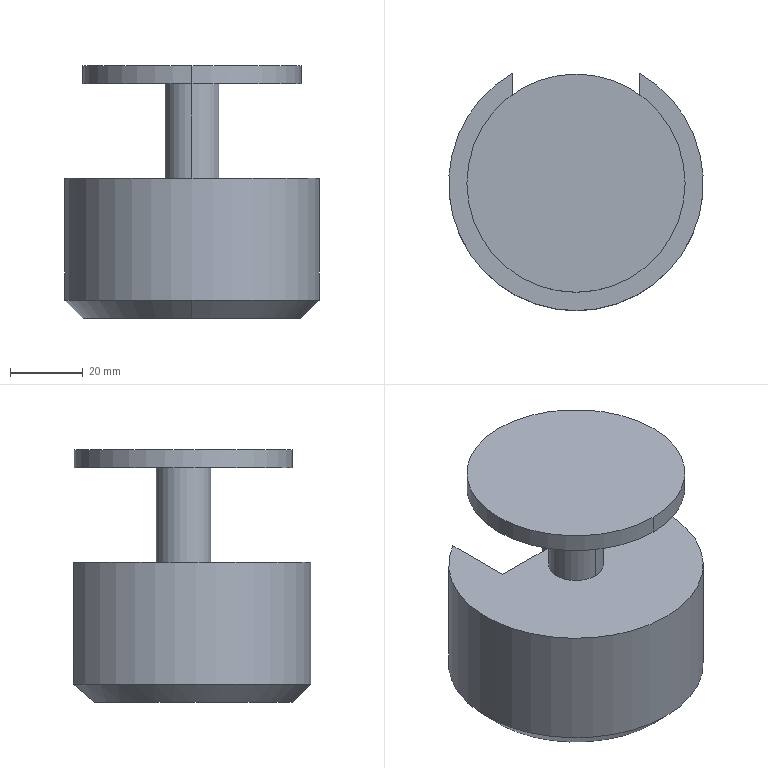Part | STEP file | ASND-0110-E63-HLTP01Clogo.sldasm-Part-213 | 1 solid | 14 faces | box 70 x 65.311 x 69.5 mm | volume 134446 mm3 | plane 7 | cylinder 5 | cone 2 | commonest cylinder face diameters 15 x2 60 x2 70 x1
STEP:
#1=CARTESIAN_POINT('',(0.,0.,0.));
#2=DIRECTION('',(0.,0.,1.));
#3=DIRECTION('',(1.,0.,0.));
#4=AXIS2_PLACEMENT_3D('',#1,#2,#3);
#5=CARTESIAN_POINT('',(320.5,-90.,-1064.2));
#6=VERTEX_POINT('',#5);
#7=CARTESIAN_POINT('',(303.,-35.633,-1064.2));
#8=VERTEX_POINT('',#7);
#9=CARTESIAN_POINT('',(320.5,-60.,-1064.2));
#10=DIRECTION('',(0.,0.,-1.));
#11=DIRECTION('',(0.,1.,0.));
#12=AXIS2_PLACEMENT_3D('',#9,#10,#11);
#13=CIRCLE('',#12,30.);
#14=CARTESIAN_POINT('',(320.5,-60.,-1064.2));
#15=DIRECTION('',(0.,0.,1.));
#16=DIRECTION('',(0.,-1.,0.));
#17=AXIS2_PLACEMENT_3D('',#14,#15,#16);
#18=CONICAL_SURFACE('',#17,30.,0.7854);
#19=CARTESIAN_POINT('',(9.425,0.));
#20=DIRECTION('',(-1.,0.));
#21=VECTOR('',#20,1.);
#22=LINE('',#19,#21);
#23=(GEOMETRIC_REPRESENTATION_CONTEXT(2)PARAMETRIC_REPRESENTATION_CONTEXT()REPRESENTATION_CONTEXT('',''));
#24=DEFINITIONAL_REPRESENTATION('',(#22),#23);
#25=PCURVE('',#18,#24);
#26=CARTESIAN_POINT('',(320.5,-60.,-1064.2));
#27=DIRECTION('',(0.,0.,-1.));
#28=DIRECTION('',(0.7071,0.7071,0.));
#29=AXIS2_PLACEMENT_3D('',#26,#27,#28);
#30=PLANE('',#29);
#31=CARTESIAN_POINT('',(0.,0.));
#32=DIRECTION('',(0.7071,-0.7071));
#33=AXIS2_PLACEMENT_2D('',#31,#32);
#34=CIRCLE('',#33,30.);
#35=(GEOMETRIC_REPRESENTATION_CONTEXT(2)PARAMETRIC_REPRESENTATION_CONTEXT()REPRESENTATION_CONTEXT('',''));
#36=DEFINITIONAL_REPRESENTATION('',(#34),#35);
#37=PCURVE('',#30,#36);
#38=SURFACE_CURVE('',#13,(#25,#37),.PCURVE_S1.);
#39=EDGE_CURVE('',#6,#8,#38,.T.);
#40=ORIENTED_EDGE('',*,*,#39,.F.);
#41=CARTESIAN_POINT('',(320.5,-95.,-1059.2));
#42=VERTEX_POINT('',#41);
#43=CARTESIAN_POINT('',(320.5,-90.,-1064.2));
#44=DIRECTION('',(0.,-0.7071,0.7071));
#45=VECTOR('',#44,1.);
#46=LINE('',#43,#45);
#47=CARTESIAN_POINT('',(6.283,0.));
#48=DIRECTION('',(0.,1.));
#49=VECTOR('',#48,1.);
#50=LINE('',#47,#49);
#51=(GEOMETRIC_REPRESENTATION_CONTEXT(2)PARAMETRIC_REPRESENTATION_CONTEXT()REPRESENTATION_CONTEXT('',''));
#52=DEFINITIONAL_REPRESENTATION('',(#50),#51);
#53=PCURVE('',#18,#52);
#54=CARTESIAN_POINT('',(320.5,-60.,-1064.2));
#55=DIRECTION('',(0.,0.,1.));
#56=DIRECTION('',(0.,-1.,0.));
#57=AXIS2_PLACEMENT_3D('',#54,#55,#56);
#58=CONICAL_SURFACE('',#57,30.,0.7854);
#59=CARTESIAN_POINT('',(0.,0.));
#60=DIRECTION('',(0.,1.));
#61=VECTOR('',#60,1.);
#62=LINE('',#59,#61);
#63=(GEOMETRIC_REPRESENTATION_CONTEXT(2)PARAMETRIC_REPRESENTATION_CONTEXT()REPRESENTATION_CONTEXT('',''));
#64=DEFINITIONAL_REPRESENTATION('',(#62),#63);
#65=PCURVE('',#58,#64);
#66=SURFACE_CURVE('',#46,(#53,#65),.PCURVE_S1.);
#67=EDGE_CURVE('',#6,#42,#66,.T.);
#68=ORIENTED_EDGE('',*,*,#67,.T.);
#69=CARTESIAN_POINT('',(303.,-29.689,-1059.2));
#70=VERTEX_POINT('',#69);
#71=CARTESIAN_POINT('',(320.5,-60.,-1059.2));
#72=DIRECTION('',(0.,0.,1.));
#73=DIRECTION('',(0.,1.,0.));
#74=AXIS2_PLACEMENT_3D('',#71,#72,#73);
#75=CIRCLE('',#74,35.);
#76=CARTESIAN_POINT('',(3.142,5.));
#77=DIRECTION('',(1.,0.));
#78=VECTOR('',#77,1.);
#79=LINE('',#76,#78);
#80=(GEOMETRIC_REPRESENTATION_CONTEXT(2)PARAMETRIC_REPRESENTATION_CONTEXT()REPRESENTATION_CONTEXT('',''));
#81=DEFINITIONAL_REPRESENTATION('',(#79),#80);
#82=PCURVE('',#18,#81);
#83=CARTESIAN_POINT('',(320.5,-60.,-1025.7));
#84=DIRECTION('',(0.,0.,-1.));
#85=DIRECTION('',(0.,1.,0.));
#86=AXIS2_PLACEMENT_3D('',#83,#84,#85);
#87=CYLINDRICAL_SURFACE('',#86,35.);
#88=CARTESIAN_POINT('',(6.283,33.5));
#89=DIRECTION('',(-1.,0.));
#90=VECTOR('',#89,1.);
#91=LINE('',#88,#90);
#92=(GEOMETRIC_REPRESENTATION_CONTEXT(2)PARAMETRIC_REPRESENTATION_CONTEXT()REPRESENTATION_CONTEXT('',''));
#93=DEFINITIONAL_REPRESENTATION('',(#91),#92);
#94=PCURVE('',#87,#93);
#95=SURFACE_CURVE('',#75,(#82,#94),.PCURVE_S1.);
#96=EDGE_CURVE('',#70,#42,#95,.T.);
#97=ORIENTED_EDGE('',*,*,#96,.F.);
#98=CARTESIAN_POINT('',(303.,-35.633,-1064.2));
#99=CARTESIAN_POINT('',(303.,-32.89,-1061.972));
#100=CARTESIAN_POINT('',(303.,-29.689,-1059.2));
#101=(BOUNDED_CURVE()B_SPLINE_CURVE(2,(#98,#99,#100),.UNSPECIFIED.,.F.,.F.)B_SPLINE_CURVE_WITH_KNOTS((3,3),(0.253,1.379),.PIECEWISE_BEZIER_KNOTS.)CURVE()GEOMETRIC_REPRESENTATION_ITEM()RATIONAL_B_SPLINE_CURVE((1.01,1.03,1.042))REPRESENTATION_ITEM(''));
#102=CARTESIAN_POINT('',(3.764,0.));
#103=CARTESIAN_POINT('',(3.763,0.06889));
#104=CARTESIAN_POINT('',(3.759,0.2073));
#105=CARTESIAN_POINT('',(3.755,0.4166));
#106=CARTESIAN_POINT('',(3.75,0.6277));
#107=CARTESIAN_POINT('',(3.745,0.8407));
#108=CARTESIAN_POINT('',(3.74,1.055));
#109=CARTESIAN_POINT('',(3.735,1.272));
#110=CARTESIAN_POINT('',(3.731,1.491));
#111=CARTESIAN_POINT('',(3.726,1.711));
#112=CARTESIAN_POINT('',(3.722,1.933));
#113=CARTESIAN_POINT('',(3.717,2.157));
#114=CARTESIAN_POINT('',(3.712,2.383));
#115=CARTESIAN_POINT('',(3.708,2.611));
#116=CARTESIAN_POINT('',(3.704,2.841));
#117=CARTESIAN_POINT('',(3.699,3.073));
#118=CARTESIAN_POINT('',(3.695,3.307));
#119=CARTESIAN_POINT('',(3.69,3.542));
#120=CARTESIAN_POINT('',(3.686,3.78));
#121=CARTESIAN_POINT('',(3.682,4.02));
#122=CARTESIAN_POINT('',(3.678,4.262));
#123=CARTESIAN_POINT('',(3.673,4.506));
#124=CARTESIAN_POINT('',(3.669,4.752));
#125=CARTESIAN_POINT('',(3.667,4.917));
#126=CARTESIAN_POINT('',(3.665,5.));
#127=B_SPLINE_CURVE_WITH_KNOTS('',3,(#102,#103,#104,#105,#106,#107,#108,#109,#110,#111,#112,#113,#114,#115,#116,#117,#118,#119,#120,#121,#122,#123,#124,#125,#126),.UNSPECIFIED.,.F.,.F.,(4,1,1,1,1,1,1,1,1,1,1,1,1,1,1,1,1,1,1,1,1,1,4),(0.253,0.3041,0.3553,0.4065,0.4577,0.5089,0.56,0.6112,0.6624,0.7136,0.7647,0.8159,0.8671,0.9183,0.9695,1.021,1.072,1.123,1.174,1.225,1.277,1.328,1.379),.QUASI_UNIFORM_KNOTS.);
#128=(GEOMETRIC_REPRESENTATION_CONTEXT(2)PARAMETRIC_REPRESENTATION_CONTEXT()REPRESENTATION_CONTEXT('',''));
#129=DEFINITIONAL_REPRESENTATION('',(#127),#128);
#130=PCURVE('',#18,#129);
#131=CARTESIAN_POINT('',(303.,-29.689,-1025.7));
#132=DIRECTION('',(1.,0.,0.));
#133=DIRECTION('',(0.,0.7071,0.7071));
#134=AXIS2_PLACEMENT_3D('',#131,#132,#133);
#135=PLANE('',#134);
#136=CARTESIAN_POINT('',(-31.427,-23.021));
#137=CARTESIAN_POINT('',(-27.911,-23.385));
#138=CARTESIAN_POINT('',(-23.688,-23.688));
#139=(BOUNDED_CURVE()B_SPLINE_CURVE(2,(#136,#137,#138),.UNSPECIFIED.,.F.,.F.)B_SPLINE_CURVE_WITH_KNOTS((3,3),(0.253,1.379),.PIECEWISE_BEZIER_KNOTS.)CURVE()GEOMETRIC_REPRESENTATION_ITEM()RATIONAL_B_SPLINE_CURVE((1.01,1.03,1.042))REPRESENTATION_ITEM(''));
#140=(GEOMETRIC_REPRESENTATION_CONTEXT(2)PARAMETRIC_REPRESENTATION_CONTEXT()REPRESENTATION_CONTEXT('',''));
#141=DEFINITIONAL_REPRESENTATION('',(#139),#140);
#142=PCURVE('',#135,#141);
#143=SURFACE_CURVE('',#101,(#130,#142),.PCURVE_S1.);
#144=EDGE_CURVE('',#8,#70,#143,.T.);
#145=ORIENTED_EDGE('',*,*,#144,.F.);
#146=EDGE_LOOP('',(#40,#68,#97,#145));
#147=FACE_BOUND('',#146,.T.);
#148=ADVANCED_FACE('',(#147),#18,.T.);
#149=CARTESIAN_POINT('',(320.5,-90.,-999.7));
#150=VERTEX_POINT('',#149);
#151=CARTESIAN_POINT('',(320.5,-30.,-999.7));
#152=VERTEX_POINT('',#151);
#153=CARTESIAN_POINT('',(320.5,-60.,-999.7));
#154=DIRECTION('',(0.,0.,1.));
#155=DIRECTION('',(0.,-1.,0.));
#156=AXIS2_PLACEMENT_3D('',#153,#154,#155);
#157=CIRCLE('',#156,30.);
#158=CARTESIAN_POINT('',(320.5,-60.,-999.7));
#159=DIRECTION('',(0.,0.,1.));
#160=DIRECTION('',(0.,-1.,0.));
#161=AXIS2_PLACEMENT_3D('',#158,#159,#160);
#162=CYLINDRICAL_SURFACE('',#161,30.);
#163=CARTESIAN_POINT('',(0.,0.));
#164=DIRECTION('',(1.,0.));
#165=VECTOR('',#164,1.);
#166=LINE('',#163,#165);
#167=(GEOMETRIC_REPRESENTATION_CONTEXT(2)PARAMETRIC_REPRESENTATION_CONTEXT()REPRESENTATION_CONTEXT('',''));
#168=DEFINITIONAL_REPRESENTATION('',(#166),#167);
#169=PCURVE('',#162,#168);
#170=CARTESIAN_POINT('',(320.5,-60.,-999.7));
#171=DIRECTION('',(0.,0.,1.));
#172=DIRECTION('',(0.7071,0.7071,0.));
#173=AXIS2_PLACEMENT_3D('',#170,#171,#172);
#174=PLANE('',#173);
#175=CARTESIAN_POINT('',(0.,0.));
#176=DIRECTION('',(-0.7071,-0.7071));
#177=AXIS2_PLACEMENT_2D('',#175,#176);
#178=CIRCLE('',#177,30.);
#179=(GEOMETRIC_REPRESENTATION_CONTEXT(2)PARAMETRIC_REPRESENTATION_CONTEXT()REPRESENTATION_CONTEXT('',''));
#180=DEFINITIONAL_REPRESENTATION('',(#178),#179);
#181=PCURVE('',#174,#180);
#182=SURFACE_CURVE('',#157,(#169,#181),.PCURVE_S1.);
#183=EDGE_CURVE('',#150,#152,#182,.T.);
#184=ORIENTED_EDGE('',*,*,#183,.T.);
#185=CARTESIAN_POINT('',(320.5,-30.,-994.7));
#186=VERTEX_POINT('',#185);
#187=CARTESIAN_POINT('',(320.5,-30.,-999.7));
#188=DIRECTION('',(0.,0.,1.));
#189=VECTOR('',#188,1.);
#190=LINE('',#187,#189);
#191=CARTESIAN_POINT('',(3.142,0.));
#192=DIRECTION('',(0.,1.));
#193=VECTOR('',#192,1.);
#194=LINE('',#191,#193);
#195=(GEOMETRIC_REPRESENTATION_CONTEXT(2)PARAMETRIC_REPRESENTATION_CONTEXT()REPRESENTATION_CONTEXT('',''));
#196=DEFINITIONAL_REPRESENTATION('',(#194),#195);
#197=PCURVE('',#162,#196);
#198=CARTESIAN_POINT('',(320.5,-60.,-999.7));
#199=DIRECTION('',(0.,0.,1.));
#200=DIRECTION('',(0.,-1.,0.));
#201=AXIS2_PLACEMENT_3D('',#198,#199,#200);
#202=CYLINDRICAL_SURFACE('',#201,30.);
#203=CARTESIAN_POINT('',(3.142,0.));
#204=DIRECTION('',(0.,1.));
#205=VECTOR('',#204,1.);
#206=LINE('',#203,#205);
#207=(GEOMETRIC_REPRESENTATION_CONTEXT(2)PARAMETRIC_REPRESENTATION_CONTEXT()REPRESENTATION_CONTEXT('',''));
#208=DEFINITIONAL_REPRESENTATION('',(#206),#207);
#209=PCURVE('',#202,#208);
#210=SURFACE_CURVE('',#190,(#197,#209),.PCURVE_S1.);
#211=EDGE_CURVE('',#152,#186,#210,.T.);
#212=ORIENTED_EDGE('',*,*,#211,.T.);
#213=CARTESIAN_POINT('',(320.5,-90.,-994.7));
#214=VERTEX_POINT('',#213);
#215=CARTESIAN_POINT('',(320.5,-60.,-994.7));
#216=DIRECTION('',(0.,0.,1.));
#217=DIRECTION('',(0.,-1.,0.));
#218=AXIS2_PLACEMENT_3D('',#215,#216,#217);
#219=CIRCLE('',#218,30.);
#220=CARTESIAN_POINT('',(0.,5.));
#221=DIRECTION('',(1.,0.));
#222=VECTOR('',#221,1.);
#223=LINE('',#220,#222);
#224=(GEOMETRIC_REPRESENTATION_CONTEXT(2)PARAMETRIC_REPRESENTATION_CONTEXT()REPRESENTATION_CONTEXT('',''));
#225=DEFINITIONAL_REPRESENTATION('',(#223),#224);
#226=PCURVE('',#162,#225);
#227=CARTESIAN_POINT('',(320.5,-60.,-994.7));
#228=DIRECTION('',(0.,0.,1.));
#229=DIRECTION('',(0.7071,0.7071,0.));
#230=AXIS2_PLACEMENT_3D('',#227,#228,#229);
#231=PLANE('',#230);
#232=CARTESIAN_POINT('',(0.,0.));
#233=DIRECTION('',(-0.7071,-0.7071));
#234=AXIS2_PLACEMENT_2D('',#232,#233);
#235=CIRCLE('',#234,30.);
#236=(GEOMETRIC_REPRESENTATION_CONTEXT(2)PARAMETRIC_REPRESENTATION_CONTEXT()REPRESENTATION_CONTEXT('',''));
#237=DEFINITIONAL_REPRESENTATION('',(#235),#236);
#238=PCURVE('',#231,#237);
#239=SURFACE_CURVE('',#219,(#226,#238),.PCURVE_S1.);
#240=EDGE_CURVE('',#214,#186,#239,.T.);
#241=ORIENTED_EDGE('',*,*,#240,.F.);
#242=CARTESIAN_POINT('',(320.5,-90.,-999.7));
#243=DIRECTION('',(0.,0.,1.));
#244=VECTOR('',#243,1.);
#245=LINE('',#242,#244);
#246=CARTESIAN_POINT('',(0.,0.));
#247=DIRECTION('',(0.,1.));
#248=VECTOR('',#247,1.);
#249=LINE('',#246,#248);
#250=(GEOMETRIC_REPRESENTATION_CONTEXT(2)PARAMETRIC_REPRESENTATION_CONTEXT()REPRESENTATION_CONTEXT('',''));
#251=DEFINITIONAL_REPRESENTATION('',(#249),#250);
#252=PCURVE('',#162,#251);
#253=CARTESIAN_POINT('',(6.283,0.));
#254=DIRECTION('',(0.,1.));
#255=VECTOR('',#254,1.);
#256=LINE('',#253,#255);
#257=(GEOMETRIC_REPRESENTATION_CONTEXT(2)PARAMETRIC_REPRESENTATION_CONTEXT()REPRESENTATION_CONTEXT('',''));
#258=DEFINITIONAL_REPRESENTATION('',(#256),#257);
#259=PCURVE('',#202,#258);
#260=SURFACE_CURVE('',#245,(#252,#259),.PCURVE_S1.);
#261=EDGE_CURVE('',#150,#214,#260,.T.);
#262=ORIENTED_EDGE('',*,*,#261,.F.);
#263=EDGE_LOOP('',(#184,#212,#241,#262));
#264=FACE_BOUND('',#263,.T.);
#265=ADVANCED_FACE('',(#264),#162,.T.);
#266=CARTESIAN_POINT('',(320.5,-67.5,-999.7));
#267=VERTEX_POINT('',#266);
#268=CARTESIAN_POINT('',(320.5,-52.5,-999.7));
#269=VERTEX_POINT('',#268);
#270=CARTESIAN_POINT('',(320.5,-60.,-999.7));
#271=DIRECTION('',(0.,0.,1.));
#272=DIRECTION('',(0.,-1.,0.));
#273=AXIS2_PLACEMENT_3D('',#270,#271,#272);
#274=CIRCLE('',#273,7.5);
#275=CARTESIAN_POINT('',(320.5,-60.,-997.7));
#276=DIRECTION('',(0.,0.,-1.));
#277=DIRECTION('',(0.,1.,0.));
#278=AXIS2_PLACEMENT_3D('',#275,#276,#277);
#279=CYLINDRICAL_SURFACE('',#278,7.5);
#280=CARTESIAN_POINT('',(3.142,2.));
#281=DIRECTION('',(-1.,0.));
#282=VECTOR('',#281,1.);
#283=LINE('',#280,#282);
#284=(GEOMETRIC_REPRESENTATION_CONTEXT(2)PARAMETRIC_REPRESENTATION_CONTEXT()REPRESENTATION_CONTEXT('',''));
#285=DEFINITIONAL_REPRESENTATION('',(#283),#284);
#286=PCURVE('',#279,#285);
#287=CARTESIAN_POINT('',(0.,0.));
#288=DIRECTION('',(-0.7071,-0.7071));
#289=AXIS2_PLACEMENT_2D('',#287,#288);
#290=CIRCLE('',#289,7.5);
#291=(GEOMETRIC_REPRESENTATION_CONTEXT(2)PARAMETRIC_REPRESENTATION_CONTEXT()REPRESENTATION_CONTEXT('',''));
#292=DEFINITIONAL_REPRESENTATION('',(#290),#291);
#293=PCURVE('',#174,#292);
#294=SURFACE_CURVE('',#274,(#286,#293),.PCURVE_S1.);
#295=EDGE_CURVE('',#267,#269,#294,.T.);
#296=ORIENTED_EDGE('',*,*,#295,.F.);
#297=CARTESIAN_POINT('',(320.5,-67.5,-1025.7));
#298=VERTEX_POINT('',#297);
#299=CARTESIAN_POINT('',(320.5,-67.5,-997.7));
#300=DIRECTION('',(0.,0.,-1.));
#301=VECTOR('',#300,1.);
#302=LINE('',#299,#301);
#303=CARTESIAN_POINT('',(3.142,0.));
#304=DIRECTION('',(0.,1.));
#305=VECTOR('',#304,1.);
#306=LINE('',#303,#305);
#307=(GEOMETRIC_REPRESENTATION_CONTEXT(2)PARAMETRIC_REPRESENTATION_CONTEXT()REPRESENTATION_CONTEXT('',''));
#308=DEFINITIONAL_REPRESENTATION('',(#306),#307);
#309=PCURVE('',#279,#308);
#310=CARTESIAN_POINT('',(320.5,-60.,-997.7));
#311=DIRECTION('',(0.,0.,-1.));
#312=DIRECTION('',(0.,1.,0.));
#313=AXIS2_PLACEMENT_3D('',#310,#311,#312);
#314=CYLINDRICAL_SURFACE('',#313,7.5);
#315=CARTESIAN_POINT('',(3.142,0.));
#316=DIRECTION('',(0.,1.));
#317=VECTOR('',#316,1.);
#318=LINE('',#315,#317);
#319=(GEOMETRIC_REPRESENTATION_CONTEXT(2)PARAMETRIC_REPRESENTATION_CONTEXT()REPRESENTATION_CONTEXT('',''));
#320=DEFINITIONAL_REPRESENTATION('',(#318),#319);
#321=PCURVE('',#314,#320);
#322=SURFACE_CURVE('',#302,(#309,#321),.PCURVE_S1.);
#323=EDGE_CURVE('',#267,#298,#322,.T.);
#324=ORIENTED_EDGE('',*,*,#323,.T.);
#325=CARTESIAN_POINT('',(320.5,-52.5,-1025.7));
#326=VERTEX_POINT('',#325);
#327=CARTESIAN_POINT('',(320.5,-60.,-1025.7));
#328=DIRECTION('',(0.,0.,1.));
#329=DIRECTION('',(0.,1.,0.));
#330=AXIS2_PLACEMENT_3D('',#327,#328,#329);
#331=CIRCLE('',#330,7.5);
#332=CARTESIAN_POINT('',(6.283,28.));
#333=DIRECTION('',(-1.,0.));
#334=VECTOR('',#333,1.);
#335=LINE('',#332,#334);
#336=(GEOMETRIC_REPRESENTATION_CONTEXT(2)PARAMETRIC_REPRESENTATION_CONTEXT()REPRESENTATION_CONTEXT('',''));
#337=DEFINITIONAL_REPRESENTATION('',(#335),#336);
#338=PCURVE('',#279,#337);
#339=CARTESIAN_POINT('',(320.5,-60.,-1025.7));
#340=DIRECTION('',(0.,0.,-1.));
#341=DIRECTION('',(0.7071,0.7071,0.));
#342=AXIS2_PLACEMENT_3D('',#339,#340,#341);
#343=PLANE('',#342);
#344=CARTESIAN_POINT('',(5.303,-5.303));
#345=CARTESIAN_POINT('',(-3.882,-14.489));
#346=CARTESIAN_POINT('',(-7.244,-1.941));
#347=CARTESIAN_POINT('',(-10.607,10.607));
#348=CARTESIAN_POINT('',(1.941,7.244));
#349=CARTESIAN_POINT('',(14.489,3.882));
#350=CARTESIAN_POINT('',(5.303,-5.303));
#351=(BOUNDED_CURVE()B_SPLINE_CURVE(2,(#344,#345,#346,#347,#348,#349,#350),.UNSPECIFIED.,.T.,.F.)B_SPLINE_CURVE_WITH_KNOTS((1,2,2,2,2,1),(-2.094,0.,2.094,4.189,6.283,8.378),.UNSPECIFIED.)CURVE()GEOMETRIC_REPRESENTATION_ITEM()RATIONAL_B_SPLINE_CURVE((1.,0.5,1.,0.5,1.,0.5,1.))REPRESENTATION_ITEM(''));
#352=(GEOMETRIC_REPRESENTATION_CONTEXT(2)PARAMETRIC_REPRESENTATION_CONTEXT()REPRESENTATION_CONTEXT('',''));
#353=DEFINITIONAL_REPRESENTATION('',(#351),#352);
#354=PCURVE('',#343,#353);
#355=SURFACE_CURVE('',#331,(#338,#354),.PCURVE_S1.);
#356=EDGE_CURVE('',#298,#326,#355,.T.);
#357=ORIENTED_EDGE('',*,*,#356,.T.);
#358=CARTESIAN_POINT('',(320.5,-52.5,-997.7));
#359=DIRECTION('',(0.,0.,-1.));
#360=VECTOR('',#359,1.);
#361=LINE('',#358,#360);
#362=CARTESIAN_POINT('',(0.,0.));
#363=DIRECTION('',(0.,1.));
#364=VECTOR('',#363,1.);
#365=LINE('',#362,#364);
#366=(GEOMETRIC_REPRESENTATION_CONTEXT(2)PARAMETRIC_REPRESENTATION_CONTEXT()REPRESENTATION_CONTEXT('',''));
#367=DEFINITIONAL_REPRESENTATION('',(#365),#366);
#368=PCURVE('',#279,#367);
#369=CARTESIAN_POINT('',(6.283,0.));
#370=DIRECTION('',(0.,1.));
#371=VECTOR('',#370,1.);
#372=LINE('',#369,#371);
#373=(GEOMETRIC_REPRESENTATION_CONTEXT(2)PARAMETRIC_REPRESENTATION_CONTEXT()REPRESENTATION_CONTEXT('',''));
#374=DEFINITIONAL_REPRESENTATION('',(#372),#373);
#375=PCURVE('',#314,#374);
#376=SURFACE_CURVE('',#361,(#368,#375),.PCURVE_S1.);
#377=EDGE_CURVE('',#269,#326,#376,.T.);
#378=ORIENTED_EDGE('',*,*,#377,.F.);
#379=EDGE_LOOP('',(#296,#324,#357,#378));
#380=FACE_BOUND('',#379,.T.);
#381=ADVANCED_FACE('',(#380),#279,.T.);
#382=CARTESIAN_POINT('',(338.,-49.,-1064.2));
#383=VERTEX_POINT('',#382);
#384=CARTESIAN_POINT('',(338.,-35.633,-1064.2));
#385=VERTEX_POINT('',#384);
#386=CARTESIAN_POINT('',(338.,-49.,-1064.2));
#387=DIRECTION('',(0.,1.,0.));
#388=VECTOR('',#387,1.);
#389=LINE('',#386,#388);
#390=CARTESIAN_POINT('',(20.153,4.596));
#391=DIRECTION('',(0.7071,-0.7071));
#392=VECTOR('',#391,1.);
#393=LINE('',#390,#392);
#394=(GEOMETRIC_REPRESENTATION_CONTEXT(2)PARAMETRIC_REPRESENTATION_CONTEXT()REPRESENTATION_CONTEXT('',''));
#395=DEFINITIONAL_REPRESENTATION('',(#393),#394);
#396=PCURVE('',#30,#395);
#397=CARTESIAN_POINT('',(338.,-29.689,-1025.7));
#398=DIRECTION('',(-1.,0.,0.));
#399=DIRECTION('',(0.,0.7071,0.7071));
#400=AXIS2_PLACEMENT_3D('',#397,#398,#399);
#401=PLANE('',#400);
#402=CARTESIAN_POINT('',(-40.878,13.569));
#403=DIRECTION('',(0.7071,0.7071));
#404=VECTOR('',#403,1.);
#405=LINE('',#402,#404);
#406=(GEOMETRIC_REPRESENTATION_CONTEXT(2)PARAMETRIC_REPRESENTATION_CONTEXT()REPRESENTATION_CONTEXT('',''));
#407=DEFINITIONAL_REPRESENTATION('',(#405),#406);
#408=PCURVE('',#401,#407);
#409=SURFACE_CURVE('',#389,(#396,#408),.PCURVE_S1.);
#410=EDGE_CURVE('',#383,#385,#409,.T.);
#411=ORIENTED_EDGE('',*,*,#410,.T.);
#412=CARTESIAN_POINT('',(320.5,-60.,-1064.2));
#413=DIRECTION('',(0.,0.,-1.));
#414=DIRECTION('',(0.,1.,0.));
#415=AXIS2_PLACEMENT_3D('',#412,#413,#414);
#416=CIRCLE('',#415,30.);
#417=CARTESIAN_POINT('',(0.,0.));
#418=DIRECTION('',(0.7071,-0.7071));
#419=AXIS2_PLACEMENT_2D('',#417,#418);
#420=CIRCLE('',#419,30.);
#421=(GEOMETRIC_REPRESENTATION_CONTEXT(2)PARAMETRIC_REPRESENTATION_CONTEXT()REPRESENTATION_CONTEXT('',''));
#422=DEFINITIONAL_REPRESENTATION('',(#420),#421);
#423=PCURVE('',#30,#422);
#424=CARTESIAN_POINT('',(3.142,0.));
#425=DIRECTION('',(-1.,0.));
#426=VECTOR('',#425,1.);
#427=LINE('',#424,#426);
#428=(GEOMETRIC_REPRESENTATION_CONTEXT(2)PARAMETRIC_REPRESENTATION_CONTEXT()REPRESENTATION_CONTEXT('',''));
#429=DEFINITIONAL_REPRESENTATION('',(#427),#428);
#430=PCURVE('',#58,#429);
#431=SURFACE_CURVE('',#416,(#423,#430),.PCURVE_S1.);
#432=EDGE_CURVE('',#385,#6,#431,.T.);
#433=ORIENTED_EDGE('',*,*,#432,.T.);
#434=ORIENTED_EDGE('',*,*,#39,.T.);
#435=CARTESIAN_POINT('',(303.,-49.,-1064.2));
#436=VERTEX_POINT('',#435);
#437=CARTESIAN_POINT('',(303.,-35.633,-1064.2));
#438=DIRECTION('',(0.,-1.,0.));
#439=VECTOR('',#438,1.);
#440=LINE('',#437,#439);
#441=CARTESIAN_POINT('',(4.856,-29.604));
#442=DIRECTION('',(-0.7071,0.7071));
#443=VECTOR('',#442,1.);
#444=LINE('',#441,#443);
#445=(GEOMETRIC_REPRESENTATION_CONTEXT(2)PARAMETRIC_REPRESENTATION_CONTEXT()REPRESENTATION_CONTEXT('',''));
#446=DEFINITIONAL_REPRESENTATION('',(#444),#445);
#447=PCURVE('',#30,#446);
#448=CARTESIAN_POINT('',(-31.427,-23.021));
#449=DIRECTION('',(-0.7071,0.7071));
#450=VECTOR('',#449,1.);
#451=LINE('',#448,#450);
#452=(GEOMETRIC_REPRESENTATION_CONTEXT(2)PARAMETRIC_REPRESENTATION_CONTEXT()REPRESENTATION_CONTEXT('',''));
#453=DEFINITIONAL_REPRESENTATION('',(#451),#452);
#454=PCURVE('',#135,#453);
#455=SURFACE_CURVE('',#440,(#447,#454),.PCURVE_S1.);
#456=EDGE_CURVE('',#8,#436,#455,.T.);
#457=ORIENTED_EDGE('',*,*,#456,.T.);
#458=CARTESIAN_POINT('',(303.,-49.,-1064.2));
#459=DIRECTION('',(1.,0.,0.));
#460=VECTOR('',#459,1.);
#461=LINE('',#458,#460);
#462=CARTESIAN_POINT('',(-4.596,-20.153));
#463=DIRECTION('',(0.7071,0.7071));
#464=VECTOR('',#463,1.);
#465=LINE('',#462,#464);
#466=(GEOMETRIC_REPRESENTATION_CONTEXT(2)PARAMETRIC_REPRESENTATION_CONTEXT()REPRESENTATION_CONTEXT('',''));
#467=DEFINITIONAL_REPRESENTATION('',(#465),#466);
#468=PCURVE('',#30,#467);
#469=CARTESIAN_POINT('',(303.,-49.,-1025.7));
#470=DIRECTION('',(0.,1.,0.));
#471=DIRECTION('',(0.7071,0.,0.7071));
#472=AXIS2_PLACEMENT_3D('',#469,#470,#471);
#473=PLANE('',#472);
#474=CARTESIAN_POINT('',(-27.224,27.224));
#475=DIRECTION('',(0.7071,0.7071));
#476=VECTOR('',#475,1.);
#477=LINE('',#474,#476);
#478=(GEOMETRIC_REPRESENTATION_CONTEXT(2)PARAMETRIC_REPRESENTATION_CONTEXT()REPRESENTATION_CONTEXT('',''));
#479=DEFINITIONAL_REPRESENTATION('',(#477),#478);
#480=PCURVE('',#473,#479);
#481=SURFACE_CURVE('',#461,(#468,#480),.PCURVE_S1.);
#482=EDGE_CURVE('',#436,#383,#481,.T.);
#483=ORIENTED_EDGE('',*,*,#482,.T.);
#484=EDGE_LOOP('',(#411,#433,#434,#457,#483));
#485=FACE_BOUND('',#484,.T.);
#486=ADVANCED_FACE('',(#485),#30,.T.);
#487=CARTESIAN_POINT('',(303.,-29.689,-1025.7));
#488=VERTEX_POINT('',#487);
#489=CARTESIAN_POINT('',(303.,-49.,-1025.7));
#490=VERTEX_POINT('',#489);
#491=CARTESIAN_POINT('',(303.,-29.689,-1025.7));
#492=DIRECTION('',(0.,-1.,0.));
#493=VECTOR('',#492,1.);
#494=LINE('',#491,#493);
#495=CARTESIAN_POINT('',(9.059,-33.807));
#496=DIRECTION('',(-0.7071,0.7071));
#497=VECTOR('',#496,1.);
#498=LINE('',#495,#497);
#499=(GEOMETRIC_REPRESENTATION_CONTEXT(2)PARAMETRIC_REPRESENTATION_CONTEXT()REPRESENTATION_CONTEXT('',''));
#500=DEFINITIONAL_REPRESENTATION('',(#498),#499);
#501=PCURVE('',#343,#500);
#502=CARTESIAN_POINT('',(0.,0.));
#503=DIRECTION('',(-0.7071,0.7071));
#504=VECTOR('',#503,1.);
#505=LINE('',#502,#504);
#506=(GEOMETRIC_REPRESENTATION_CONTEXT(2)PARAMETRIC_REPRESENTATION_CONTEXT()REPRESENTATION_CONTEXT('',''));
#507=DEFINITIONAL_REPRESENTATION('',(#505),#506);
#508=PCURVE('',#135,#507);
#509=SURFACE_CURVE('',#494,(#501,#508),.PCURVE_S1.);
#510=EDGE_CURVE('',#488,#490,#509,.T.);
#511=ORIENTED_EDGE('',*,*,#510,.F.);
#512=CARTESIAN_POINT('',(338.,-29.689,-1025.7));
#513=VERTEX_POINT('',#512);
#514=CARTESIAN_POINT('',(320.5,-60.,-1025.7));
#515=DIRECTION('',(0.,0.,-1.));
#516=DIRECTION('',(0.,1.,0.));
#517=AXIS2_PLACEMENT_3D('',#514,#515,#516);
#518=CIRCLE('',#517,35.);
#519=CARTESIAN_POINT('',(0.,0.));
#520=DIRECTION('',(0.7071,-0.7071));
#521=AXIS2_PLACEMENT_2D('',#519,#520);
#522=CIRCLE('',#521,35.);
#523=(GEOMETRIC_REPRESENTATION_CONTEXT(2)PARAMETRIC_REPRESENTATION_CONTEXT()REPRESENTATION_CONTEXT('',''));
#524=DEFINITIONAL_REPRESENTATION('',(#522),#523);
#525=PCURVE('',#343,#524);
#526=CARTESIAN_POINT('',(0.,0.));
#527=DIRECTION('',(1.,0.));
#528=VECTOR('',#527,1.);
#529=LINE('',#526,#528);
#530=(GEOMETRIC_REPRESENTATION_CONTEXT(2)PARAMETRIC_REPRESENTATION_CONTEXT()REPRESENTATION_CONTEXT('',''));
#531=DEFINITIONAL_REPRESENTATION('',(#529),#530);
#532=PCURVE('',#87,#531);
#533=SURFACE_CURVE('',#518,(#525,#532),.PCURVE_S1.);
#534=EDGE_CURVE('',#513,#488,#533,.T.);
#535=ORIENTED_EDGE('',*,*,#534,.F.);
#536=CARTESIAN_POINT('',(338.,-49.,-1025.7));
#537=VERTEX_POINT('',#536);
#538=CARTESIAN_POINT('',(338.,-49.,-1025.7));
#539=DIRECTION('',(0.,1.,0.));
#540=VECTOR('',#539,1.);
#541=LINE('',#538,#540);
#542=CARTESIAN_POINT('',(20.153,4.596));
#543=DIRECTION('',(0.7071,-0.7071));
#544=VECTOR('',#543,1.);
#545=LINE('',#542,#544);
#546=(GEOMETRIC_REPRESENTATION_CONTEXT(2)PARAMETRIC_REPRESENTATION_CONTEXT()REPRESENTATION_CONTEXT('',''));
#547=DEFINITIONAL_REPRESENTATION('',(#545),#546);
#548=PCURVE('',#343,#547);
#549=CARTESIAN_POINT('',(-13.655,-13.655));
#550=DIRECTION('',(0.7071,0.7071));
#551=VECTOR('',#550,1.);
#552=LINE('',#549,#551);
#553=(GEOMETRIC_REPRESENTATION_CONTEXT(2)PARAMETRIC_REPRESENTATION_CONTEXT()REPRESENTATION_CONTEXT('',''));
#554=DEFINITIONAL_REPRESENTATION('',(#552),#553);
#555=PCURVE('',#401,#554);
#556=SURFACE_CURVE('',#541,(#548,#555),.PCURVE_S1.);
#557=EDGE_CURVE('',#537,#513,#556,.T.);
#558=ORIENTED_EDGE('',*,*,#557,.F.);
#559=CARTESIAN_POINT('',(303.,-49.,-1025.7));
#560=DIRECTION('',(1.,0.,0.));
#561=VECTOR('',#560,1.);
#562=LINE('',#559,#561);
#563=CARTESIAN_POINT('',(-4.596,-20.153));
#564=DIRECTION('',(0.7071,0.7071));
#565=VECTOR('',#564,1.);
#566=LINE('',#563,#565);
#567=(GEOMETRIC_REPRESENTATION_CONTEXT(2)PARAMETRIC_REPRESENTATION_CONTEXT()REPRESENTATION_CONTEXT('',''));
#568=DEFINITIONAL_REPRESENTATION('',(#566),#567);
#569=PCURVE('',#343,#568);
#570=CARTESIAN_POINT('',(0.,0.));
#571=DIRECTION('',(0.7071,0.7071));
#572=VECTOR('',#571,1.);
#573=LINE('',#570,#572);
#574=(GEOMETRIC_REPRESENTATION_CONTEXT(2)PARAMETRIC_REPRESENTATION_CONTEXT()REPRESENTATION_CONTEXT('',''));
#575=DEFINITIONAL_REPRESENTATION('',(#573),#574);
#576=PCURVE('',#473,#575);
#577=SURFACE_CURVE('',#562,(#569,#576),.PCURVE_S1.);
#578=EDGE_CURVE('',#490,#537,#577,.T.);
#579=ORIENTED_EDGE('',*,*,#578,.F.);
#580=EDGE_LOOP('',(#511,#535,#558,#579));
#581=FACE_BOUND('',#580,.T.);
#582=CARTESIAN_POINT('',(320.5,-60.,-1025.7));
#583=DIRECTION('',(0.,0.,1.));
#584=DIRECTION('',(0.,1.,0.));
#585=AXIS2_PLACEMENT_3D('',#582,#583,#584);
#586=CIRCLE('',#585,7.5);
#587=CARTESIAN_POINT('',(5.303,-5.303));
#588=CARTESIAN_POINT('',(-3.882,-14.489));
#589=CARTESIAN_POINT('',(-7.244,-1.941));
#590=CARTESIAN_POINT('',(-10.607,10.607));
#591=CARTESIAN_POINT('',(1.941,7.244));
#592=CARTESIAN_POINT('',(14.489,3.882));
#593=CARTESIAN_POINT('',(5.303,-5.303));
#594=(BOUNDED_CURVE()B_SPLINE_CURVE(2,(#587,#588,#589,#590,#591,#592,#593),.UNSPECIFIED.,.T.,.F.)B_SPLINE_CURVE_WITH_KNOTS((1,2,2,2,2,1),(-2.094,0.,2.094,4.189,6.283,8.378),.UNSPECIFIED.)CURVE()GEOMETRIC_REPRESENTATION_ITEM()RATIONAL_B_SPLINE_CURVE((1.,0.5,1.,0.5,1.,0.5,1.))REPRESENTATION_ITEM(''));
#595=(GEOMETRIC_REPRESENTATION_CONTEXT(2)PARAMETRIC_REPRESENTATION_CONTEXT()REPRESENTATION_CONTEXT('',''));
#596=DEFINITIONAL_REPRESENTATION('',(#594),#595);
#597=PCURVE('',#343,#596);
#598=CARTESIAN_POINT('',(6.283,28.));
#599=DIRECTION('',(-1.,0.));
#600=VECTOR('',#599,1.);
#601=LINE('',#598,#600);
#602=(GEOMETRIC_REPRESENTATION_CONTEXT(2)PARAMETRIC_REPRESENTATION_CONTEXT()REPRESENTATION_CONTEXT('',''));
#603=DEFINITIONAL_REPRESENTATION('',(#601),#602);
#604=PCURVE('',#314,#603);
#605=SURFACE_CURVE('',#586,(#597,#604),.PCURVE_S1.);
#606=EDGE_CURVE('',#326,#298,#605,.T.);
#607=ORIENTED_EDGE('',*,*,#606,.F.);
#608=ORIENTED_EDGE('',*,*,#356,.F.);
#609=EDGE_LOOP('',(#607,#608));
#610=FACE_BOUND('',#609,.T.);
#611=ADVANCED_FACE('',(#581,#610),#343,.F.);
#612=ORIENTED_EDGE('',*,*,#323,.F.);
#613=CARTESIAN_POINT('',(320.5,-60.,-999.7));
#614=DIRECTION('',(0.,0.,1.));
#615=DIRECTION('',(0.,-1.,0.));
#616=AXIS2_PLACEMENT_3D('',#613,#614,#615);
#617=CIRCLE('',#616,7.5);
#618=CARTESIAN_POINT('',(9.425,2.));
#619=DIRECTION('',(-1.,0.));
#620=VECTOR('',#619,1.);
#621=LINE('',#618,#620);
#622=(GEOMETRIC_REPRESENTATION_CONTEXT(2)PARAMETRIC_REPRESENTATION_CONTEXT()REPRESENTATION_CONTEXT('',''));
#623=DEFINITIONAL_REPRESENTATION('',(#621),#622);
#624=PCURVE('',#314,#623);
#625=CARTESIAN_POINT('',(0.,0.));
#626=DIRECTION('',(-0.7071,-0.7071));
#627=AXIS2_PLACEMENT_2D('',#625,#626);
#628=CIRCLE('',#627,7.5);
#629=(GEOMETRIC_REPRESENTATION_CONTEXT(2)PARAMETRIC_REPRESENTATION_CONTEXT()REPRESENTATION_CONTEXT('',''));
#630=DEFINITIONAL_REPRESENTATION('',(#628),#629);
#631=PCURVE('',#174,#630);
#632=SURFACE_CURVE('',#617,(#624,#631),.PCURVE_S1.);
#633=EDGE_CURVE('',#269,#267,#632,.T.);
#634=ORIENTED_EDGE('',*,*,#633,.F.);
#635=ORIENTED_EDGE('',*,*,#377,.T.);
#636=ORIENTED_EDGE('',*,*,#606,.T.);
#637=EDGE_LOOP('',(#612,#634,#635,#636));
#638=FACE_BOUND('',#637,.T.);
#639=ADVANCED_FACE('',(#638),#314,.T.);
#640=CARTESIAN_POINT('',(338.,-49.,-1025.7));
#641=DIRECTION('',(0.,0.,-1.));
#642=VECTOR('',#641,1.);
#643=LINE('',#640,#642);
#644=CARTESIAN_POINT('',(24.749,24.749));
#645=DIRECTION('',(-0.7071,0.7071));
#646=VECTOR('',#645,1.);
#647=LINE('',#644,#646);
#648=(GEOMETRIC_REPRESENTATION_CONTEXT(2)PARAMETRIC_REPRESENTATION_CONTEXT()REPRESENTATION_CONTEXT('',''));
#649=DEFINITIONAL_REPRESENTATION('',(#647),#648);
#650=PCURVE('',#473,#649);
#651=CARTESIAN_POINT('',(-13.655,-13.655));
#652=DIRECTION('',(-0.7071,0.7071));
#653=VECTOR('',#652,1.);
#654=LINE('',#651,#653);
#655=(GEOMETRIC_REPRESENTATION_CONTEXT(2)PARAMETRIC_REPRESENTATION_CONTEXT()REPRESENTATION_CONTEXT('',''));
#656=DEFINITIONAL_REPRESENTATION('',(#654),#655);
#657=PCURVE('',#401,#656);
#658=SURFACE_CURVE('',#643,(#650,#657),.PCURVE_S1.);
#659=EDGE_CURVE('',#537,#383,#658,.T.);
#660=ORIENTED_EDGE('',*,*,#659,.T.);
#661=ORIENTED_EDGE('',*,*,#482,.F.);
#662=CARTESIAN_POINT('',(303.,-49.,-1025.7));
#663=DIRECTION('',(0.,0.,-1.));
#664=VECTOR('',#663,1.);
#665=LINE('',#662,#664);
#666=CARTESIAN_POINT('',(0.,0.));
#667=DIRECTION('',(-0.7071,0.7071));
#668=VECTOR('',#667,1.);
#669=LINE('',#666,#668);
#670=(GEOMETRIC_REPRESENTATION_CONTEXT(2)PARAMETRIC_REPRESENTATION_CONTEXT()REPRESENTATION_CONTEXT('',''));
#671=DEFINITIONAL_REPRESENTATION('',(#669),#670);
#672=PCURVE('',#473,#671);
#673=CARTESIAN_POINT('',(-13.655,13.655));
#674=DIRECTION('',(-0.7071,-0.7071));
#675=VECTOR('',#674,1.);
#676=LINE('',#673,#675);
#677=(GEOMETRIC_REPRESENTATION_CONTEXT(2)PARAMETRIC_REPRESENTATION_CONTEXT()REPRESENTATION_CONTEXT('',''));
#678=DEFINITIONAL_REPRESENTATION('',(#676),#677);
#679=PCURVE('',#135,#678);
#680=SURFACE_CURVE('',#665,(#672,#679),.PCURVE_S1.);
#681=EDGE_CURVE('',#490,#436,#680,.T.);
#682=ORIENTED_EDGE('',*,*,#681,.F.);
#683=ORIENTED_EDGE('',*,*,#578,.T.);
#684=EDGE_LOOP('',(#660,#661,#682,#683));
#685=FACE_BOUND('',#684,.T.);
#686=ADVANCED_FACE('',(#685),#473,.T.);
#687=ORIENTED_EDGE('',*,*,#456,.F.);
#688=ORIENTED_EDGE('',*,*,#144,.T.);
#689=CARTESIAN_POINT('',(303.,-29.689,-1025.7));
#690=DIRECTION('',(0.,0.,-1.));
#691=VECTOR('',#690,1.);
#692=LINE('',#689,#691);
#693=CARTESIAN_POINT('',(0.,0.));
#694=DIRECTION('',(-0.7071,-0.7071));
#695=VECTOR('',#694,1.);
#696=LINE('',#693,#695);
#697=(GEOMETRIC_REPRESENTATION_CONTEXT(2)PARAMETRIC_REPRESENTATION_CONTEXT()REPRESENTATION_CONTEXT('',''));
#698=DEFINITIONAL_REPRESENTATION('',(#696),#697);
#699=PCURVE('',#135,#698);
#700=CARTESIAN_POINT('',(5.76,0.));
#701=DIRECTION('',(0.,1.));
#702=VECTOR('',#701,1.);
#703=LINE('',#700,#702);
#704=(GEOMETRIC_REPRESENTATION_CONTEXT(2)PARAMETRIC_REPRESENTATION_CONTEXT()REPRESENTATION_CONTEXT('',''));
#705=DEFINITIONAL_REPRESENTATION('',(#703),#704);
#706=PCURVE('',#87,#705);
#707=SURFACE_CURVE('',#692,(#699,#706),.PCURVE_S1.);
#708=EDGE_CURVE('',#488,#70,#707,.T.);
#709=ORIENTED_EDGE('',*,*,#708,.F.);
#710=ORIENTED_EDGE('',*,*,#510,.T.);
#711=ORIENTED_EDGE('',*,*,#681,.T.);
#712=EDGE_LOOP('',(#687,#688,#709,#710,#711));
#713=FACE_BOUND('',#712,.T.);
#714=ADVANCED_FACE('',(#713),#135,.T.);
#715=CARTESIAN_POINT('',(338.,-29.689,-1059.2));
#716=VERTEX_POINT('',#715);
#717=CARTESIAN_POINT('',(338.,-29.689,-1025.7));
#718=DIRECTION('',(0.,0.,-1.));
#719=VECTOR('',#718,1.);
#720=LINE('',#717,#719);
#721=CARTESIAN_POINT('',(0.,0.));
#722=DIRECTION('',(-0.7071,0.7071));
#723=VECTOR('',#722,1.);
#724=LINE('',#721,#723);
#725=(GEOMETRIC_REPRESENTATION_CONTEXT(2)PARAMETRIC_REPRESENTATION_CONTEXT()REPRESENTATION_CONTEXT('',''));
#726=DEFINITIONAL_REPRESENTATION('',(#724),#725);
#727=PCURVE('',#401,#726);
#728=CARTESIAN_POINT('',(0.5236,0.));
#729=DIRECTION('',(0.,1.));
#730=VECTOR('',#729,1.);
#731=LINE('',#728,#730);
#732=(GEOMETRIC_REPRESENTATION_CONTEXT(2)PARAMETRIC_REPRESENTATION_CONTEXT()REPRESENTATION_CONTEXT('',''));
#733=DEFINITIONAL_REPRESENTATION('',(#731),#732);
#734=PCURVE('',#87,#733);
#735=SURFACE_CURVE('',#720,(#727,#734),.PCURVE_S1.);
#736=EDGE_CURVE('',#513,#716,#735,.T.);
#737=ORIENTED_EDGE('',*,*,#736,.T.);
#738=CARTESIAN_POINT('',(338.,-29.689,-1059.2));
#739=CARTESIAN_POINT('',(338.,-32.89,-1061.972));
#740=CARTESIAN_POINT('',(338.,-35.633,-1064.2));
#741=(BOUNDED_CURVE()B_SPLINE_CURVE(2,(#738,#739,#740),.UNSPECIFIED.,.F.,.F.)B_SPLINE_CURVE_WITH_KNOTS((3,3),(4.613,5.739),.PIECEWISE_BEZIER_KNOTS.)CURVE()GEOMETRIC_REPRESENTATION_ITEM()RATIONAL_B_SPLINE_CURVE((1.042,1.03,1.01))REPRESENTATION_ITEM(''));
#742=CARTESIAN_POINT('',(-23.688,23.688));
#743=CARTESIAN_POINT('',(-27.911,23.385));
#744=CARTESIAN_POINT('',(-31.427,23.021));
#745=(BOUNDED_CURVE()B_SPLINE_CURVE(2,(#742,#743,#744),.UNSPECIFIED.,.F.,.F.)B_SPLINE_CURVE_WITH_KNOTS((3,3),(4.613,5.739),.PIECEWISE_BEZIER_KNOTS.)CURVE()GEOMETRIC_REPRESENTATION_ITEM()RATIONAL_B_SPLINE_CURVE((1.042,1.03,1.01))REPRESENTATION_ITEM(''));
#746=(GEOMETRIC_REPRESENTATION_CONTEXT(2)PARAMETRIC_REPRESENTATION_CONTEXT()REPRESENTATION_CONTEXT('',''));
#747=DEFINITIONAL_REPRESENTATION('',(#745),#746);
#748=PCURVE('',#401,#747);
#749=CARTESIAN_POINT('',(2.618,5.));
#750=CARTESIAN_POINT('',(2.617,4.917));
#751=CARTESIAN_POINT('',(2.614,4.752));
#752=CARTESIAN_POINT('',(2.61,4.506));
#753=CARTESIAN_POINT('',(2.606,4.262));
#754=CARTESIAN_POINT('',(2.601,4.02));
#755=CARTESIAN_POINT('',(2.597,3.78));
#756=CARTESIAN_POINT('',(2.593,3.542));
#757=CARTESIAN_POINT('',(2.588,3.307));
#758=CARTESIAN_POINT('',(2.584,3.073));
#759=CARTESIAN_POINT('',(2.58,2.841));
#760=CARTESIAN_POINT('',(2.575,2.611));
#761=CARTESIAN_POINT('',(2.571,2.383));
#762=CARTESIAN_POINT('',(2.566,2.157));
#763=CARTESIAN_POINT('',(2.562,1.933));
#764=CARTESIAN_POINT('',(2.557,1.711));
#765=CARTESIAN_POINT('',(2.552,1.491));
#766=CARTESIAN_POINT('',(2.548,1.272));
#767=CARTESIAN_POINT('',(2.543,1.055));
#768=CARTESIAN_POINT('',(2.538,0.8407));
#769=CARTESIAN_POINT('',(2.533,0.6277));
#770=CARTESIAN_POINT('',(2.529,0.4166));
#771=CARTESIAN_POINT('',(2.524,0.2073));
#772=CARTESIAN_POINT('',(2.52,0.06889));
#773=CARTESIAN_POINT('',(2.519,0.));
#774=B_SPLINE_CURVE_WITH_KNOTS('',3,(#749,#750,#751,#752,#753,#754,#755,#756,#757,#758,#759,#760,#761,#762,#763,#764,#765,#766,#767,#768,#769,#770,#771,#772,#773),.UNSPECIFIED.,.F.,.F.,(4,1,1,1,1,1,1,1,1,1,1,1,1,1,1,1,1,1,1,1,1,1,4),(4.613,4.664,4.715,4.766,4.817,4.869,4.92,4.971,5.022,5.073,5.124,5.176,5.227,5.278,5.329,5.38,5.431,5.483,5.534,5.585,5.636,5.687,5.739),.QUASI_UNIFORM_KNOTS.);
#775=(GEOMETRIC_REPRESENTATION_CONTEXT(2)PARAMETRIC_REPRESENTATION_CONTEXT()REPRESENTATION_CONTEXT('',''));
#776=DEFINITIONAL_REPRESENTATION('',(#774),#775);
#777=PCURVE('',#58,#776);
#778=SURFACE_CURVE('',#741,(#748,#777),.PCURVE_S1.);
#779=EDGE_CURVE('',#716,#385,#778,.T.);
#780=ORIENTED_EDGE('',*,*,#779,.T.);
#781=ORIENTED_EDGE('',*,*,#410,.F.);
#782=ORIENTED_EDGE('',*,*,#659,.F.);
#783=ORIENTED_EDGE('',*,*,#557,.T.);
#784=EDGE_LOOP('',(#737,#780,#781,#782,#783));
#785=FACE_BOUND('',#784,.T.);
#786=ADVANCED_FACE('',(#785),#401,.T.);
#787=ORIENTED_EDGE('',*,*,#183,.F.);
#788=CARTESIAN_POINT('',(320.5,-60.,-999.7));
#789=DIRECTION('',(0.,0.,1.));
#790=DIRECTION('',(0.,-1.,0.));
#791=AXIS2_PLACEMENT_3D('',#788,#789,#790);
#792=CIRCLE('',#791,30.);
#793=CARTESIAN_POINT('',(0.,0.));
#794=DIRECTION('',(-0.7071,-0.7071));
#795=AXIS2_PLACEMENT_2D('',#793,#794);
#796=CIRCLE('',#795,30.);
#797=(GEOMETRIC_REPRESENTATION_CONTEXT(2)PARAMETRIC_REPRESENTATION_CONTEXT()REPRESENTATION_CONTEXT('',''));
#798=DEFINITIONAL_REPRESENTATION('',(#796),#797);
#799=PCURVE('',#174,#798);
#800=CARTESIAN_POINT('',(0.,0.));
#801=DIRECTION('',(1.,0.));
#802=VECTOR('',#801,1.);
#803=LINE('',#800,#802);
#804=(GEOMETRIC_REPRESENTATION_CONTEXT(2)PARAMETRIC_REPRESENTATION_CONTEXT()REPRESENTATION_CONTEXT('',''));
#805=DEFINITIONAL_REPRESENTATION('',(#803),#804);
#806=PCURVE('',#202,#805);
#807=SURFACE_CURVE('',#792,(#799,#806),.PCURVE_S1.);
#808=EDGE_CURVE('',#152,#150,#807,.T.);
#809=ORIENTED_EDGE('',*,*,#808,.F.);
#810=EDGE_LOOP('',(#787,#809));
#811=FACE_BOUND('',#810,.T.);
#812=ORIENTED_EDGE('',*,*,#633,.T.);
#813=ORIENTED_EDGE('',*,*,#295,.T.);
#814=EDGE_LOOP('',(#812,#813));
#815=FACE_BOUND('',#814,.T.);
#816=ADVANCED_FACE('',(#811,#815),#174,.F.);
#817=ORIENTED_EDGE('',*,*,#211,.F.);
#818=ORIENTED_EDGE('',*,*,#808,.T.);
#819=ORIENTED_EDGE('',*,*,#261,.T.);
#820=CARTESIAN_POINT('',(320.5,-60.,-994.7));
#821=DIRECTION('',(0.,0.,1.));
#822=DIRECTION('',(0.,-1.,0.));
#823=AXIS2_PLACEMENT_3D('',#820,#821,#822);
#824=CIRCLE('',#823,30.);
#825=CARTESIAN_POINT('',(0.,5.));
#826=DIRECTION('',(1.,0.));
#827=VECTOR('',#826,1.);
#828=LINE('',#825,#827);
#829=(GEOMETRIC_REPRESENTATION_CONTEXT(2)PARAMETRIC_REPRESENTATION_CONTEXT()REPRESENTATION_CONTEXT('',''));
#830=DEFINITIONAL_REPRESENTATION('',(#828),#829);
#831=PCURVE('',#202,#830);
#832=CARTESIAN_POINT('',(0.,0.));
#833=DIRECTION('',(-0.7071,-0.7071));
#834=AXIS2_PLACEMENT_2D('',#832,#833);
#835=CIRCLE('',#834,30.);
#836=(GEOMETRIC_REPRESENTATION_CONTEXT(2)PARAMETRIC_REPRESENTATION_CONTEXT()REPRESENTATION_CONTEXT('',''));
#837=DEFINITIONAL_REPRESENTATION('',(#835),#836);
#838=PCURVE('',#231,#837);
#839=SURFACE_CURVE('',#824,(#831,#838),.PCURVE_S1.);
#840=EDGE_CURVE('',#186,#214,#839,.T.);
#841=ORIENTED_EDGE('',*,*,#840,.F.);
#842=EDGE_LOOP('',(#817,#818,#819,#841));
#843=FACE_BOUND('',#842,.T.);
#844=ADVANCED_FACE('',(#843),#202,.T.);
#845=ORIENTED_EDGE('',*,*,#240,.T.);
#846=ORIENTED_EDGE('',*,*,#840,.T.);
#847=EDGE_LOOP('',(#845,#846));
#848=FACE_BOUND('',#847,.T.);
#849=ADVANCED_FACE('',(#848),#231,.T.);
#850=ORIENTED_EDGE('',*,*,#708,.T.);
#851=ORIENTED_EDGE('',*,*,#96,.T.);
#852=CARTESIAN_POINT('',(320.5,-60.,-1059.2));
#853=DIRECTION('',(0.,0.,1.));
#854=DIRECTION('',(0.,1.,0.));
#855=AXIS2_PLACEMENT_3D('',#852,#853,#854);
#856=CIRCLE('',#855,35.);
#857=CARTESIAN_POINT('',(6.283,33.5));
#858=DIRECTION('',(-1.,0.));
#859=VECTOR('',#858,1.);
#860=LINE('',#857,#859);
#861=(GEOMETRIC_REPRESENTATION_CONTEXT(2)PARAMETRIC_REPRESENTATION_CONTEXT()REPRESENTATION_CONTEXT('',''));
#862=DEFINITIONAL_REPRESENTATION('',(#860),#861);
#863=PCURVE('',#87,#862);
#864=CARTESIAN_POINT('',(-3.142,5.));
#865=DIRECTION('',(1.,0.));
#866=VECTOR('',#865,1.);
#867=LINE('',#864,#866);
#868=(GEOMETRIC_REPRESENTATION_CONTEXT(2)PARAMETRIC_REPRESENTATION_CONTEXT()REPRESENTATION_CONTEXT('',''));
#869=DEFINITIONAL_REPRESENTATION('',(#867),#868);
#870=PCURVE('',#58,#869);
#871=SURFACE_CURVE('',#856,(#863,#870),.PCURVE_S1.);
#872=EDGE_CURVE('',#42,#716,#871,.T.);
#873=ORIENTED_EDGE('',*,*,#872,.T.);
#874=ORIENTED_EDGE('',*,*,#736,.F.);
#875=ORIENTED_EDGE('',*,*,#534,.T.);
#876=EDGE_LOOP('',(#850,#851,#873,#874,#875));
#877=FACE_BOUND('',#876,.T.);
#878=ADVANCED_FACE('',(#877),#87,.T.);
#879=ORIENTED_EDGE('',*,*,#67,.F.);
#880=ORIENTED_EDGE('',*,*,#432,.F.);
#881=ORIENTED_EDGE('',*,*,#779,.F.);
#882=ORIENTED_EDGE('',*,*,#872,.F.);
#883=EDGE_LOOP('',(#879,#880,#881,#882));
#884=FACE_BOUND('',#883,.T.);
#885=ADVANCED_FACE('',(#884),#58,.T.);
#886=CLOSED_SHELL('',(#148,#265,#381,#486,#611,#639,#686,#714,#786,#816,#844,#849,#878,#885));
#887=MANIFOLD_SOLID_BREP('',#886);
#888=(LENGTH_UNIT()NAMED_UNIT(*)SI_UNIT(.MILLI.,.METRE.));
#889=UNCERTAINTY_MEASURE_WITH_UNIT(LENGTH_MEASURE(0.0000001),#888,'','');
#890=(NAMED_UNIT(*)PLANE_ANGLE_UNIT()SI_UNIT($,.RADIAN.));
#891=(NAMED_UNIT(*)SI_UNIT($,.STERADIAN.)SOLID_ANGLE_UNIT());
#892=(GEOMETRIC_REPRESENTATION_CONTEXT(3)GLOBAL_UNCERTAINTY_ASSIGNED_CONTEXT((#889))GLOBAL_UNIT_ASSIGNED_CONTEXT((#888,#890,#891))REPRESENTATION_CONTEXT('',''));
#893=ADVANCED_BREP_SHAPE_REPRESENTATION('',(#4,#887),#892);